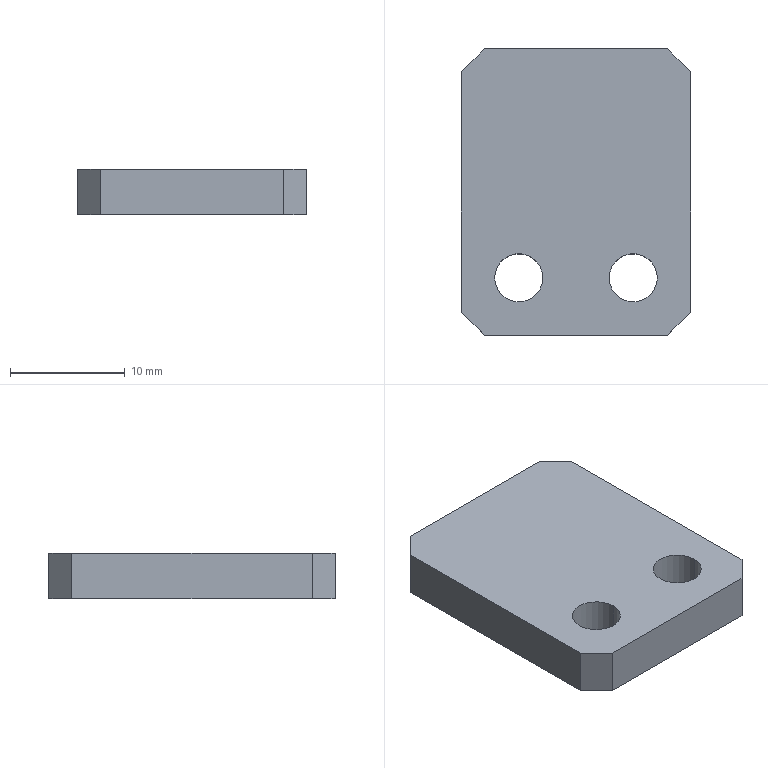Part | STEP file | PN_0085 Mount electronic clip slider stop plate | 1 solid | 14 faces | box 20 x 25 x 4 mm | volume 1857 mm3 | plane 10 | cylinder 4 | commonest cylinder face diameters 4.2 x4
STEP:
#1=CARTESIAN_POINT('',(0.,0.,0.));
#2=DIRECTION('',(0.,0.,1.));
#3=DIRECTION('',(1.,0.,0.));
#4=AXIS2_PLACEMENT_3D('',#1,#2,#3);
#5=CARTESIAN_POINT('',(-2.9,-7.5,0.));
#6=VERTEX_POINT('',#5);
#7=CARTESIAN_POINT('',(-2.9,-7.5,4.));
#8=VERTEX_POINT('',#7);
#9=CARTESIAN_POINT('',(-2.9,-7.5,4.));
#10=DIRECTION('',(0.,0.,1.));
#11=VECTOR('',#10,1.);
#12=LINE('',#9,#11);
#13=CARTESIAN_POINT('',(-5.,-7.5,4.));
#14=DIRECTION('',(0.,0.,1.));
#15=DIRECTION('',(1.,0.,0.));
#16=AXIS2_PLACEMENT_3D('',#13,#14,#15);
#17=CYLINDRICAL_SURFACE('',#16,2.1);
#18=CARTESIAN_POINT('',(6.283,0.));
#19=DIRECTION('',(0.,1.));
#20=VECTOR('',#19,1.);
#21=LINE('',#18,#20);
#22=(GEOMETRIC_REPRESENTATION_CONTEXT(2)PARAMETRIC_REPRESENTATION_CONTEXT()REPRESENTATION_CONTEXT('',''));
#23=DEFINITIONAL_REPRESENTATION('',(#21),#22);
#24=PCURVE('',#17,#23);
#25=CARTESIAN_POINT('',(-5.,-7.5,4.));
#26=DIRECTION('',(0.,0.,1.));
#27=DIRECTION('',(1.,0.,0.));
#28=AXIS2_PLACEMENT_3D('',#25,#26,#27);
#29=CYLINDRICAL_SURFACE('',#28,2.1);
#30=CARTESIAN_POINT('',(0.,0.));
#31=DIRECTION('',(0.,1.));
#32=VECTOR('',#31,1.);
#33=LINE('',#30,#32);
#34=(GEOMETRIC_REPRESENTATION_CONTEXT(2)PARAMETRIC_REPRESENTATION_CONTEXT()REPRESENTATION_CONTEXT('',''));
#35=DEFINITIONAL_REPRESENTATION('',(#33),#34);
#36=PCURVE('',#29,#35);
#37=SURFACE_CURVE('',#12,(#24,#36),.PCURVE_S1.);
#38=EDGE_CURVE('',#6,#8,#37,.T.);
#39=ORIENTED_EDGE('',*,*,#38,.T.);
#40=CARTESIAN_POINT('',(-7.1,-7.5,4.));
#41=VERTEX_POINT('',#40);
#42=CARTESIAN_POINT('',(-5.,-7.5,4.));
#43=DIRECTION('',(0.,0.,1.));
#44=DIRECTION('',(1.,0.,0.));
#45=AXIS2_PLACEMENT_3D('',#42,#43,#44);
#46=CIRCLE('',#45,2.1);
#47=CARTESIAN_POINT('',(0.,0.));
#48=DIRECTION('',(1.,0.));
#49=VECTOR('',#48,1.);
#50=LINE('',#47,#49);
#51=(GEOMETRIC_REPRESENTATION_CONTEXT(2)PARAMETRIC_REPRESENTATION_CONTEXT()REPRESENTATION_CONTEXT('',''));
#52=DEFINITIONAL_REPRESENTATION('',(#50),#51);
#53=PCURVE('',#17,#52);
#54=CARTESIAN_POINT('',(0.,0.,4.));
#55=DIRECTION('',(0.,0.,-1.));
#56=DIRECTION('',(-1.,0.,0.));
#57=AXIS2_PLACEMENT_3D('',#54,#55,#56);
#58=PLANE('',#57);
#59=CARTESIAN_POINT('',(2.9,-7.5));
#60=CARTESIAN_POINT('',(2.9,-3.863));
#61=CARTESIAN_POINT('',(6.05,-5.681));
#62=CARTESIAN_POINT('',(9.2,-7.5));
#63=CARTESIAN_POINT('',(6.05,-9.319));
#64=CARTESIAN_POINT('',(2.9,-11.137));
#65=CARTESIAN_POINT('',(2.9,-7.5));
#66=(BOUNDED_CURVE()B_SPLINE_CURVE(2,(#59,#60,#61,#62,#63,#64,#65),.UNSPECIFIED.,.T.,.F.)B_SPLINE_CURVE_WITH_KNOTS((1,2,2,2,2,1),(-2.094,0.,2.094,4.189,6.283,8.378),.UNSPECIFIED.)CURVE()GEOMETRIC_REPRESENTATION_ITEM()RATIONAL_B_SPLINE_CURVE((1.,0.5,1.,0.5,1.,0.5,1.))REPRESENTATION_ITEM(''));
#67=(GEOMETRIC_REPRESENTATION_CONTEXT(2)PARAMETRIC_REPRESENTATION_CONTEXT()REPRESENTATION_CONTEXT('',''));
#68=DEFINITIONAL_REPRESENTATION('',(#66),#67);
#69=PCURVE('',#58,#68);
#70=SURFACE_CURVE('',#46,(#53,#69),.PCURVE_S1.);
#71=EDGE_CURVE('',#41,#8,#70,.T.);
#72=ORIENTED_EDGE('',*,*,#71,.F.);
#73=CARTESIAN_POINT('',(-7.1,-7.5,0.));
#74=VERTEX_POINT('',#73);
#75=CARTESIAN_POINT('',(-7.1,-7.5,4.));
#76=DIRECTION('',(0.,0.,1.));
#77=VECTOR('',#76,1.);
#78=LINE('',#75,#77);
#79=CARTESIAN_POINT('',(3.142,0.));
#80=DIRECTION('',(0.,1.));
#81=VECTOR('',#80,1.);
#82=LINE('',#79,#81);
#83=(GEOMETRIC_REPRESENTATION_CONTEXT(2)PARAMETRIC_REPRESENTATION_CONTEXT()REPRESENTATION_CONTEXT('',''));
#84=DEFINITIONAL_REPRESENTATION('',(#82),#83);
#85=PCURVE('',#17,#84);
#86=CARTESIAN_POINT('',(3.142,0.));
#87=DIRECTION('',(0.,1.));
#88=VECTOR('',#87,1.);
#89=LINE('',#86,#88);
#90=(GEOMETRIC_REPRESENTATION_CONTEXT(2)PARAMETRIC_REPRESENTATION_CONTEXT()REPRESENTATION_CONTEXT('',''));
#91=DEFINITIONAL_REPRESENTATION('',(#89),#90);
#92=PCURVE('',#29,#91);
#93=SURFACE_CURVE('',#78,(#85,#92),.PCURVE_S1.);
#94=EDGE_CURVE('',#74,#41,#93,.T.);
#95=ORIENTED_EDGE('',*,*,#94,.F.);
#96=CARTESIAN_POINT('',(-5.,-7.5,0.));
#97=DIRECTION('',(0.,0.,-1.));
#98=DIRECTION('',(-1.,0.,0.));
#99=AXIS2_PLACEMENT_3D('',#96,#97,#98);
#100=CIRCLE('',#99,2.1);
#101=CARTESIAN_POINT('',(9.425,-4.));
#102=DIRECTION('',(-1.,0.));
#103=VECTOR('',#102,1.);
#104=LINE('',#101,#103);
#105=(GEOMETRIC_REPRESENTATION_CONTEXT(2)PARAMETRIC_REPRESENTATION_CONTEXT()REPRESENTATION_CONTEXT('',''));
#106=DEFINITIONAL_REPRESENTATION('',(#104),#105);
#107=PCURVE('',#17,#106);
#108=CARTESIAN_POINT('',(0.,0.,0.));
#109=DIRECTION('',(0.,0.,-1.));
#110=DIRECTION('',(-1.,0.,0.));
#111=AXIS2_PLACEMENT_3D('',#108,#109,#110);
#112=PLANE('',#111);
#113=CARTESIAN_POINT('',(5.,-7.5));
#114=DIRECTION('',(1.,0.));
#115=AXIS2_PLACEMENT_2D('',#113,#114);
#116=CIRCLE('',#115,2.1);
#117=(GEOMETRIC_REPRESENTATION_CONTEXT(2)PARAMETRIC_REPRESENTATION_CONTEXT()REPRESENTATION_CONTEXT('',''));
#118=DEFINITIONAL_REPRESENTATION('',(#116),#117);
#119=PCURVE('',#112,#118);
#120=SURFACE_CURVE('',#100,(#107,#119),.PCURVE_S1.);
#121=EDGE_CURVE('',#6,#74,#120,.T.);
#122=ORIENTED_EDGE('',*,*,#121,.F.);
#123=EDGE_LOOP('',(#39,#72,#95,#122));
#124=FACE_BOUND('',#123,.F.);
#125=ADVANCED_FACE('',(#124),#17,.F.);
#126=CARTESIAN_POINT('',(7.1,-7.5,0.));
#127=VERTEX_POINT('',#126);
#128=CARTESIAN_POINT('',(7.1,-7.5,4.));
#129=VERTEX_POINT('',#128);
#130=CARTESIAN_POINT('',(7.1,-7.5,4.));
#131=DIRECTION('',(0.,0.,1.));
#132=VECTOR('',#131,1.);
#133=LINE('',#130,#132);
#134=CARTESIAN_POINT('',(5.,-7.5,4.));
#135=DIRECTION('',(0.,0.,1.));
#136=DIRECTION('',(1.,0.,0.));
#137=AXIS2_PLACEMENT_3D('',#134,#135,#136);
#138=CYLINDRICAL_SURFACE('',#137,2.1);
#139=CARTESIAN_POINT('',(6.283,0.));
#140=DIRECTION('',(0.,1.));
#141=VECTOR('',#140,1.);
#142=LINE('',#139,#141);
#143=(GEOMETRIC_REPRESENTATION_CONTEXT(2)PARAMETRIC_REPRESENTATION_CONTEXT()REPRESENTATION_CONTEXT('',''));
#144=DEFINITIONAL_REPRESENTATION('',(#142),#143);
#145=PCURVE('',#138,#144);
#146=CARTESIAN_POINT('',(5.,-7.5,4.));
#147=DIRECTION('',(0.,0.,1.));
#148=DIRECTION('',(1.,0.,0.));
#149=AXIS2_PLACEMENT_3D('',#146,#147,#148);
#150=CYLINDRICAL_SURFACE('',#149,2.1);
#151=CARTESIAN_POINT('',(0.,0.));
#152=DIRECTION('',(0.,1.));
#153=VECTOR('',#152,1.);
#154=LINE('',#151,#153);
#155=(GEOMETRIC_REPRESENTATION_CONTEXT(2)PARAMETRIC_REPRESENTATION_CONTEXT()REPRESENTATION_CONTEXT('',''));
#156=DEFINITIONAL_REPRESENTATION('',(#154),#155);
#157=PCURVE('',#150,#156);
#158=SURFACE_CURVE('',#133,(#145,#157),.PCURVE_S1.);
#159=EDGE_CURVE('',#127,#129,#158,.T.);
#160=ORIENTED_EDGE('',*,*,#159,.T.);
#161=CARTESIAN_POINT('',(2.9,-7.5,4.));
#162=VERTEX_POINT('',#161);
#163=CARTESIAN_POINT('',(5.,-7.5,4.));
#164=DIRECTION('',(0.,0.,1.));
#165=DIRECTION('',(1.,0.,0.));
#166=AXIS2_PLACEMENT_3D('',#163,#164,#165);
#167=CIRCLE('',#166,2.1);
#168=CARTESIAN_POINT('',(0.,0.));
#169=DIRECTION('',(1.,0.));
#170=VECTOR('',#169,1.);
#171=LINE('',#168,#170);
#172=(GEOMETRIC_REPRESENTATION_CONTEXT(2)PARAMETRIC_REPRESENTATION_CONTEXT()REPRESENTATION_CONTEXT('',''));
#173=DEFINITIONAL_REPRESENTATION('',(#171),#172);
#174=PCURVE('',#138,#173);
#175=CARTESIAN_POINT('',(-7.1,-7.5));
#176=CARTESIAN_POINT('',(-7.1,-3.863));
#177=CARTESIAN_POINT('',(-3.95,-5.681));
#178=CARTESIAN_POINT('',(-0.8,-7.5));
#179=CARTESIAN_POINT('',(-3.95,-9.319));
#180=CARTESIAN_POINT('',(-7.1,-11.137));
#181=CARTESIAN_POINT('',(-7.1,-7.5));
#182=(BOUNDED_CURVE()B_SPLINE_CURVE(2,(#175,#176,#177,#178,#179,#180,#181),.UNSPECIFIED.,.T.,.F.)B_SPLINE_CURVE_WITH_KNOTS((1,2,2,2,2,1),(-2.094,0.,2.094,4.189,6.283,8.378),.UNSPECIFIED.)CURVE()GEOMETRIC_REPRESENTATION_ITEM()RATIONAL_B_SPLINE_CURVE((1.,0.5,1.,0.5,1.,0.5,1.))REPRESENTATION_ITEM(''));
#183=(GEOMETRIC_REPRESENTATION_CONTEXT(2)PARAMETRIC_REPRESENTATION_CONTEXT()REPRESENTATION_CONTEXT('',''));
#184=DEFINITIONAL_REPRESENTATION('',(#182),#183);
#185=PCURVE('',#58,#184);
#186=SURFACE_CURVE('',#167,(#174,#185),.PCURVE_S1.);
#187=EDGE_CURVE('',#162,#129,#186,.T.);
#188=ORIENTED_EDGE('',*,*,#187,.F.);
#189=CARTESIAN_POINT('',(2.9,-7.5,0.));
#190=VERTEX_POINT('',#189);
#191=CARTESIAN_POINT('',(2.9,-7.5,4.));
#192=DIRECTION('',(0.,0.,1.));
#193=VECTOR('',#192,1.);
#194=LINE('',#191,#193);
#195=CARTESIAN_POINT('',(3.142,0.));
#196=DIRECTION('',(0.,1.));
#197=VECTOR('',#196,1.);
#198=LINE('',#195,#197);
#199=(GEOMETRIC_REPRESENTATION_CONTEXT(2)PARAMETRIC_REPRESENTATION_CONTEXT()REPRESENTATION_CONTEXT('',''));
#200=DEFINITIONAL_REPRESENTATION('',(#198),#199);
#201=PCURVE('',#138,#200);
#202=CARTESIAN_POINT('',(3.142,0.));
#203=DIRECTION('',(0.,1.));
#204=VECTOR('',#203,1.);
#205=LINE('',#202,#204);
#206=(GEOMETRIC_REPRESENTATION_CONTEXT(2)PARAMETRIC_REPRESENTATION_CONTEXT()REPRESENTATION_CONTEXT('',''));
#207=DEFINITIONAL_REPRESENTATION('',(#205),#206);
#208=PCURVE('',#150,#207);
#209=SURFACE_CURVE('',#194,(#201,#208),.PCURVE_S1.);
#210=EDGE_CURVE('',#190,#162,#209,.T.);
#211=ORIENTED_EDGE('',*,*,#210,.F.);
#212=CARTESIAN_POINT('',(5.,-7.5,0.));
#213=DIRECTION('',(0.,0.,-1.));
#214=DIRECTION('',(-1.,0.,0.));
#215=AXIS2_PLACEMENT_3D('',#212,#213,#214);
#216=CIRCLE('',#215,2.1);
#217=CARTESIAN_POINT('',(9.425,-4.));
#218=DIRECTION('',(-1.,0.));
#219=VECTOR('',#218,1.);
#220=LINE('',#217,#219);
#221=(GEOMETRIC_REPRESENTATION_CONTEXT(2)PARAMETRIC_REPRESENTATION_CONTEXT()REPRESENTATION_CONTEXT('',''));
#222=DEFINITIONAL_REPRESENTATION('',(#220),#221);
#223=PCURVE('',#138,#222);
#224=CARTESIAN_POINT('',(-5.,-7.5));
#225=DIRECTION('',(1.,0.));
#226=AXIS2_PLACEMENT_2D('',#224,#225);
#227=CIRCLE('',#226,2.1);
#228=(GEOMETRIC_REPRESENTATION_CONTEXT(2)PARAMETRIC_REPRESENTATION_CONTEXT()REPRESENTATION_CONTEXT('',''));
#229=DEFINITIONAL_REPRESENTATION('',(#227),#228);
#230=PCURVE('',#112,#229);
#231=SURFACE_CURVE('',#216,(#223,#230),.PCURVE_S1.);
#232=EDGE_CURVE('',#127,#190,#231,.T.);
#233=ORIENTED_EDGE('',*,*,#232,.F.);
#234=EDGE_LOOP('',(#160,#188,#211,#233));
#235=FACE_BOUND('',#234,.F.);
#236=ADVANCED_FACE('',(#235),#138,.F.);
#237=CARTESIAN_POINT('',(10.,-10.5,4.));
#238=VERTEX_POINT('',#237);
#239=CARTESIAN_POINT('',(10.,10.5,4.));
#240=VERTEX_POINT('',#239);
#241=CARTESIAN_POINT('',(10.,-12.5,4.));
#242=DIRECTION('',(0.,1.,0.));
#243=VECTOR('',#242,1.);
#244=LINE('',#241,#243);
#245=CARTESIAN_POINT('',(10.,-12.5,4.));
#246=DIRECTION('',(-1.,0.,0.));
#247=DIRECTION('',(0.,0.,1.));
#248=AXIS2_PLACEMENT_3D('',#245,#246,#247);
#249=PLANE('',#248);
#250=CARTESIAN_POINT('',(0.,0.));
#251=DIRECTION('',(0.,1.));
#252=VECTOR('',#251,1.);
#253=LINE('',#250,#252);
#254=(GEOMETRIC_REPRESENTATION_CONTEXT(2)PARAMETRIC_REPRESENTATION_CONTEXT()REPRESENTATION_CONTEXT('',''));
#255=DEFINITIONAL_REPRESENTATION('',(#253),#254);
#256=PCURVE('',#249,#255);
#257=CARTESIAN_POINT('',(-10.,-12.5));
#258=DIRECTION('',(0.,1.));
#259=VECTOR('',#258,1.);
#260=LINE('',#257,#259);
#261=(GEOMETRIC_REPRESENTATION_CONTEXT(2)PARAMETRIC_REPRESENTATION_CONTEXT()REPRESENTATION_CONTEXT('',''));
#262=DEFINITIONAL_REPRESENTATION('',(#260),#261);
#263=PCURVE('',#58,#262);
#264=SURFACE_CURVE('',#244,(#256,#263),.PCURVE_S1.);
#265=EDGE_CURVE('',#238,#240,#264,.T.);
#266=ORIENTED_EDGE('',*,*,#265,.F.);
#267=CARTESIAN_POINT('',(10.,-10.5,0.));
#268=VERTEX_POINT('',#267);
#269=CARTESIAN_POINT('',(10.,-10.5,4.));
#270=DIRECTION('',(0.,0.,-1.));
#271=VECTOR('',#270,1.);
#272=LINE('',#269,#271);
#273=CARTESIAN_POINT('',(0.,2.));
#274=DIRECTION('',(-1.,0.));
#275=VECTOR('',#274,1.);
#276=LINE('',#273,#275);
#277=(GEOMETRIC_REPRESENTATION_CONTEXT(2)PARAMETRIC_REPRESENTATION_CONTEXT()REPRESENTATION_CONTEXT('',''));
#278=DEFINITIONAL_REPRESENTATION('',(#276),#277);
#279=PCURVE('',#249,#278);
#280=CARTESIAN_POINT('',(10.,-10.5,4.));
#281=DIRECTION('',(-0.7071,0.7071,0.));
#282=DIRECTION('',(0.,0.,-1.));
#283=AXIS2_PLACEMENT_3D('',#280,#281,#282);
#284=PLANE('',#283);
#285=CARTESIAN_POINT('',(0.,0.));
#286=DIRECTION('',(1.,0.));
#287=VECTOR('',#286,1.);
#288=LINE('',#285,#287);
#289=(GEOMETRIC_REPRESENTATION_CONTEXT(2)PARAMETRIC_REPRESENTATION_CONTEXT()REPRESENTATION_CONTEXT('',''));
#290=DEFINITIONAL_REPRESENTATION('',(#288),#289);
#291=PCURVE('',#284,#290);
#292=SURFACE_CURVE('',#272,(#279,#291),.PCURVE_S1.);
#293=EDGE_CURVE('',#238,#268,#292,.T.);
#294=ORIENTED_EDGE('',*,*,#293,.T.);
#295=CARTESIAN_POINT('',(10.,10.5,0.));
#296=VERTEX_POINT('',#295);
#297=CARTESIAN_POINT('',(10.,-12.5,0.));
#298=DIRECTION('',(0.,1.,0.));
#299=VECTOR('',#298,1.);
#300=LINE('',#297,#299);
#301=CARTESIAN_POINT('',(-4.,0.));
#302=DIRECTION('',(0.,1.));
#303=VECTOR('',#302,1.);
#304=LINE('',#301,#303);
#305=(GEOMETRIC_REPRESENTATION_CONTEXT(2)PARAMETRIC_REPRESENTATION_CONTEXT()REPRESENTATION_CONTEXT('',''));
#306=DEFINITIONAL_REPRESENTATION('',(#304),#305);
#307=PCURVE('',#249,#306);
#308=CARTESIAN_POINT('',(-10.,-12.5));
#309=DIRECTION('',(0.,1.));
#310=VECTOR('',#309,1.);
#311=LINE('',#308,#310);
#312=(GEOMETRIC_REPRESENTATION_CONTEXT(2)PARAMETRIC_REPRESENTATION_CONTEXT()REPRESENTATION_CONTEXT('',''));
#313=DEFINITIONAL_REPRESENTATION('',(#311),#312);
#314=PCURVE('',#112,#313);
#315=SURFACE_CURVE('',#300,(#307,#314),.PCURVE_S1.);
#316=EDGE_CURVE('',#268,#296,#315,.T.);
#317=ORIENTED_EDGE('',*,*,#316,.T.);
#318=CARTESIAN_POINT('',(10.,10.5,4.));
#319=DIRECTION('',(0.,0.,1.));
#320=VECTOR('',#319,1.);
#321=LINE('',#318,#320);
#322=CARTESIAN_POINT('',(0.,23.));
#323=DIRECTION('',(1.,0.));
#324=VECTOR('',#323,1.);
#325=LINE('',#322,#324);
#326=(GEOMETRIC_REPRESENTATION_CONTEXT(2)PARAMETRIC_REPRESENTATION_CONTEXT()REPRESENTATION_CONTEXT('',''));
#327=DEFINITIONAL_REPRESENTATION('',(#325),#326);
#328=PCURVE('',#249,#327);
#329=CARTESIAN_POINT('',(8.,12.5,4.));
#330=DIRECTION('',(-0.7071,-0.7071,0.));
#331=DIRECTION('',(0.,0.,-1.));
#332=AXIS2_PLACEMENT_3D('',#329,#330,#331);
#333=PLANE('',#332);
#334=CARTESIAN_POINT('',(0.,2.828));
#335=DIRECTION('',(-1.,0.));
#336=VECTOR('',#335,1.);
#337=LINE('',#334,#336);
#338=(GEOMETRIC_REPRESENTATION_CONTEXT(2)PARAMETRIC_REPRESENTATION_CONTEXT()REPRESENTATION_CONTEXT('',''));
#339=DEFINITIONAL_REPRESENTATION('',(#337),#338);
#340=PCURVE('',#333,#339);
#341=SURFACE_CURVE('',#321,(#328,#340),.PCURVE_S1.);
#342=EDGE_CURVE('',#296,#240,#341,.T.);
#343=ORIENTED_EDGE('',*,*,#342,.T.);
#344=EDGE_LOOP('',(#266,#294,#317,#343));
#345=FACE_BOUND('',#344,.T.);
#346=ADVANCED_FACE('',(#345),#249,.F.);
#347=CARTESIAN_POINT('',(8.,12.5,4.));
#348=VERTEX_POINT('',#347);
#349=CARTESIAN_POINT('',(-8.,12.5,4.));
#350=VERTEX_POINT('',#349);
#351=CARTESIAN_POINT('',(-10.,12.5,4.));
#352=DIRECTION('',(-1.,0.,0.));
#353=VECTOR('',#352,1.);
#354=LINE('',#351,#353);
#355=CARTESIAN_POINT('',(-10.,12.5,4.));
#356=DIRECTION('',(0.,-1.,0.));
#357=DIRECTION('',(0.,0.,-1.));
#358=AXIS2_PLACEMENT_3D('',#355,#356,#357);
#359=PLANE('',#358);
#360=CARTESIAN_POINT('',(0.,0.));
#361=DIRECTION('',(0.,-1.));
#362=VECTOR('',#361,1.);
#363=LINE('',#360,#362);
#364=(GEOMETRIC_REPRESENTATION_CONTEXT(2)PARAMETRIC_REPRESENTATION_CONTEXT()REPRESENTATION_CONTEXT('',''));
#365=DEFINITIONAL_REPRESENTATION('',(#363),#364);
#366=PCURVE('',#359,#365);
#367=CARTESIAN_POINT('',(10.,12.5));
#368=DIRECTION('',(1.,0.));
#369=VECTOR('',#368,1.);
#370=LINE('',#367,#369);
#371=(GEOMETRIC_REPRESENTATION_CONTEXT(2)PARAMETRIC_REPRESENTATION_CONTEXT()REPRESENTATION_CONTEXT('',''));
#372=DEFINITIONAL_REPRESENTATION('',(#370),#371);
#373=PCURVE('',#58,#372);
#374=SURFACE_CURVE('',#354,(#366,#373),.PCURVE_S1.);
#375=EDGE_CURVE('',#348,#350,#374,.T.);
#376=ORIENTED_EDGE('',*,*,#375,.F.);
#377=CARTESIAN_POINT('',(8.,12.5,0.));
#378=VERTEX_POINT('',#377);
#379=CARTESIAN_POINT('',(8.,12.5,4.));
#380=DIRECTION('',(0.,0.,-1.));
#381=VECTOR('',#380,1.);
#382=LINE('',#379,#381);
#383=CARTESIAN_POINT('',(0.,18.));
#384=DIRECTION('',(1.,0.));
#385=VECTOR('',#384,1.);
#386=LINE('',#383,#385);
#387=(GEOMETRIC_REPRESENTATION_CONTEXT(2)PARAMETRIC_REPRESENTATION_CONTEXT()REPRESENTATION_CONTEXT('',''));
#388=DEFINITIONAL_REPRESENTATION('',(#386),#387);
#389=PCURVE('',#359,#388);
#390=CARTESIAN_POINT('',(0.,0.));
#391=DIRECTION('',(1.,0.));
#392=VECTOR('',#391,1.);
#393=LINE('',#390,#392);
#394=(GEOMETRIC_REPRESENTATION_CONTEXT(2)PARAMETRIC_REPRESENTATION_CONTEXT()REPRESENTATION_CONTEXT('',''));
#395=DEFINITIONAL_REPRESENTATION('',(#393),#394);
#396=PCURVE('',#333,#395);
#397=SURFACE_CURVE('',#382,(#389,#396),.PCURVE_S1.);
#398=EDGE_CURVE('',#348,#378,#397,.T.);
#399=ORIENTED_EDGE('',*,*,#398,.T.);
#400=CARTESIAN_POINT('',(-8.,12.5,0.));
#401=VERTEX_POINT('',#400);
#402=CARTESIAN_POINT('',(-10.,12.5,0.));
#403=DIRECTION('',(-1.,0.,0.));
#404=VECTOR('',#403,1.);
#405=LINE('',#402,#404);
#406=CARTESIAN_POINT('',(4.,0.));
#407=DIRECTION('',(0.,-1.));
#408=VECTOR('',#407,1.);
#409=LINE('',#406,#408);
#410=(GEOMETRIC_REPRESENTATION_CONTEXT(2)PARAMETRIC_REPRESENTATION_CONTEXT()REPRESENTATION_CONTEXT('',''));
#411=DEFINITIONAL_REPRESENTATION('',(#409),#410);
#412=PCURVE('',#359,#411);
#413=CARTESIAN_POINT('',(10.,12.5));
#414=DIRECTION('',(1.,0.));
#415=VECTOR('',#414,1.);
#416=LINE('',#413,#415);
#417=(GEOMETRIC_REPRESENTATION_CONTEXT(2)PARAMETRIC_REPRESENTATION_CONTEXT()REPRESENTATION_CONTEXT('',''));
#418=DEFINITIONAL_REPRESENTATION('',(#416),#417);
#419=PCURVE('',#112,#418);
#420=SURFACE_CURVE('',#405,(#412,#419),.PCURVE_S1.);
#421=EDGE_CURVE('',#378,#401,#420,.T.);
#422=ORIENTED_EDGE('',*,*,#421,.T.);
#423=CARTESIAN_POINT('',(-8.,12.5,4.));
#424=DIRECTION('',(0.,0.,1.));
#425=VECTOR('',#424,1.);
#426=LINE('',#423,#425);
#427=CARTESIAN_POINT('',(0.,2.));
#428=DIRECTION('',(-1.,0.));
#429=VECTOR('',#428,1.);
#430=LINE('',#427,#429);
#431=(GEOMETRIC_REPRESENTATION_CONTEXT(2)PARAMETRIC_REPRESENTATION_CONTEXT()REPRESENTATION_CONTEXT('',''));
#432=DEFINITIONAL_REPRESENTATION('',(#430),#431);
#433=PCURVE('',#359,#432);
#434=CARTESIAN_POINT('',(-10.,10.5,4.));
#435=DIRECTION('',(0.7071,-0.7071,0.));
#436=DIRECTION('',(0.,0.,-1.));
#437=AXIS2_PLACEMENT_3D('',#434,#435,#436);
#438=PLANE('',#437);
#439=CARTESIAN_POINT('',(0.,2.828));
#440=DIRECTION('',(-1.,0.));
#441=VECTOR('',#440,1.);
#442=LINE('',#439,#441);
#443=(GEOMETRIC_REPRESENTATION_CONTEXT(2)PARAMETRIC_REPRESENTATION_CONTEXT()REPRESENTATION_CONTEXT('',''));
#444=DEFINITIONAL_REPRESENTATION('',(#442),#443);
#445=PCURVE('',#438,#444);
#446=SURFACE_CURVE('',#426,(#433,#445),.PCURVE_S1.);
#447=EDGE_CURVE('',#401,#350,#446,.T.);
#448=ORIENTED_EDGE('',*,*,#447,.T.);
#449=EDGE_LOOP('',(#376,#399,#422,#448));
#450=FACE_BOUND('',#449,.T.);
#451=ADVANCED_FACE('',(#450),#359,.F.);
#452=CARTESIAN_POINT('',(-10.,10.5,0.));
#453=VERTEX_POINT('',#452);
#454=CARTESIAN_POINT('',(-10.,-10.5,0.));
#455=VERTEX_POINT('',#454);
#456=CARTESIAN_POINT('',(-10.,-12.5,0.));
#457=DIRECTION('',(0.,-1.,0.));
#458=VECTOR('',#457,1.);
#459=LINE('',#456,#458);
#460=CARTESIAN_POINT('',(-10.,-12.5,4.));
#461=DIRECTION('',(1.,0.,0.));
#462=DIRECTION('',(0.,0.,-1.));
#463=AXIS2_PLACEMENT_3D('',#460,#461,#462);
#464=PLANE('',#463);
#465=CARTESIAN_POINT('',(4.,0.));
#466=DIRECTION('',(0.,-1.));
#467=VECTOR('',#466,1.);
#468=LINE('',#465,#467);
#469=(GEOMETRIC_REPRESENTATION_CONTEXT(2)PARAMETRIC_REPRESENTATION_CONTEXT()REPRESENTATION_CONTEXT('',''));
#470=DEFINITIONAL_REPRESENTATION('',(#468),#469);
#471=PCURVE('',#464,#470);
#472=CARTESIAN_POINT('',(10.,-12.5));
#473=DIRECTION('',(0.,-1.));
#474=VECTOR('',#473,1.);
#475=LINE('',#472,#474);
#476=(GEOMETRIC_REPRESENTATION_CONTEXT(2)PARAMETRIC_REPRESENTATION_CONTEXT()REPRESENTATION_CONTEXT('',''));
#477=DEFINITIONAL_REPRESENTATION('',(#475),#476);
#478=PCURVE('',#112,#477);
#479=SURFACE_CURVE('',#459,(#471,#478),.PCURVE_S1.);
#480=EDGE_CURVE('',#453,#455,#479,.T.);
#481=ORIENTED_EDGE('',*,*,#480,.T.);
#482=CARTESIAN_POINT('',(-10.,-10.5,4.));
#483=VERTEX_POINT('',#482);
#484=CARTESIAN_POINT('',(-10.,-10.5,4.));
#485=DIRECTION('',(0.,0.,1.));
#486=VECTOR('',#485,1.);
#487=LINE('',#484,#486);
#488=CARTESIAN_POINT('',(0.,2.));
#489=DIRECTION('',(-1.,0.));
#490=VECTOR('',#489,1.);
#491=LINE('',#488,#490);
#492=(GEOMETRIC_REPRESENTATION_CONTEXT(2)PARAMETRIC_REPRESENTATION_CONTEXT()REPRESENTATION_CONTEXT('',''));
#493=DEFINITIONAL_REPRESENTATION('',(#491),#492);
#494=PCURVE('',#464,#493);
#495=CARTESIAN_POINT('',(-8.,-12.5,4.));
#496=DIRECTION('',(0.7071,0.7071,0.));
#497=DIRECTION('',(0.,0.,-1.));
#498=AXIS2_PLACEMENT_3D('',#495,#496,#497);
#499=PLANE('',#498);
#500=CARTESIAN_POINT('',(0.,2.828));
#501=DIRECTION('',(-1.,0.));
#502=VECTOR('',#501,1.);
#503=LINE('',#500,#502);
#504=(GEOMETRIC_REPRESENTATION_CONTEXT(2)PARAMETRIC_REPRESENTATION_CONTEXT()REPRESENTATION_CONTEXT('',''));
#505=DEFINITIONAL_REPRESENTATION('',(#503),#504);
#506=PCURVE('',#499,#505);
#507=SURFACE_CURVE('',#487,(#494,#506),.PCURVE_S1.);
#508=EDGE_CURVE('',#455,#483,#507,.T.);
#509=ORIENTED_EDGE('',*,*,#508,.T.);
#510=CARTESIAN_POINT('',(-10.,10.5,4.));
#511=VERTEX_POINT('',#510);
#512=CARTESIAN_POINT('',(-10.,-12.5,4.));
#513=DIRECTION('',(0.,-1.,0.));
#514=VECTOR('',#513,1.);
#515=LINE('',#512,#514);
#516=CARTESIAN_POINT('',(0.,0.));
#517=DIRECTION('',(0.,-1.));
#518=VECTOR('',#517,1.);
#519=LINE('',#516,#518);
#520=(GEOMETRIC_REPRESENTATION_CONTEXT(2)PARAMETRIC_REPRESENTATION_CONTEXT()REPRESENTATION_CONTEXT('',''));
#521=DEFINITIONAL_REPRESENTATION('',(#519),#520);
#522=PCURVE('',#464,#521);
#523=CARTESIAN_POINT('',(10.,-12.5));
#524=DIRECTION('',(0.,-1.));
#525=VECTOR('',#524,1.);
#526=LINE('',#523,#525);
#527=(GEOMETRIC_REPRESENTATION_CONTEXT(2)PARAMETRIC_REPRESENTATION_CONTEXT()REPRESENTATION_CONTEXT('',''));
#528=DEFINITIONAL_REPRESENTATION('',(#526),#527);
#529=PCURVE('',#58,#528);
#530=SURFACE_CURVE('',#515,(#522,#529),.PCURVE_S1.);
#531=EDGE_CURVE('',#511,#483,#530,.T.);
#532=ORIENTED_EDGE('',*,*,#531,.F.);
#533=CARTESIAN_POINT('',(-10.,10.5,4.));
#534=DIRECTION('',(0.,0.,-1.));
#535=VECTOR('',#534,1.);
#536=LINE('',#533,#535);
#537=CARTESIAN_POINT('',(0.,23.));
#538=DIRECTION('',(1.,0.));
#539=VECTOR('',#538,1.);
#540=LINE('',#537,#539);
#541=(GEOMETRIC_REPRESENTATION_CONTEXT(2)PARAMETRIC_REPRESENTATION_CONTEXT()REPRESENTATION_CONTEXT('',''));
#542=DEFINITIONAL_REPRESENTATION('',(#540),#541);
#543=PCURVE('',#464,#542);
#544=CARTESIAN_POINT('',(0.,0.));
#545=DIRECTION('',(1.,0.));
#546=VECTOR('',#545,1.);
#547=LINE('',#544,#546);
#548=(GEOMETRIC_REPRESENTATION_CONTEXT(2)PARAMETRIC_REPRESENTATION_CONTEXT()REPRESENTATION_CONTEXT('',''));
#549=DEFINITIONAL_REPRESENTATION('',(#547),#548);
#550=PCURVE('',#438,#549);
#551=SURFACE_CURVE('',#536,(#543,#550),.PCURVE_S1.);
#552=EDGE_CURVE('',#511,#453,#551,.T.);
#553=ORIENTED_EDGE('',*,*,#552,.T.);
#554=EDGE_LOOP('',(#481,#509,#532,#553));
#555=FACE_BOUND('',#554,.T.);
#556=ADVANCED_FACE('',(#555),#464,.F.);
#557=CARTESIAN_POINT('',(-8.,-12.5,0.));
#558=VERTEX_POINT('',#557);
#559=CARTESIAN_POINT('',(8.,-12.5,0.));
#560=VERTEX_POINT('',#559);
#561=CARTESIAN_POINT('',(-10.,-12.5,0.));
#562=DIRECTION('',(1.,0.,0.));
#563=VECTOR('',#562,1.);
#564=LINE('',#561,#563);
#565=CARTESIAN_POINT('',(-10.,-12.5,4.));
#566=DIRECTION('',(0.,1.,0.));
#567=DIRECTION('',(0.,0.,1.));
#568=AXIS2_PLACEMENT_3D('',#565,#566,#567);
#569=PLANE('',#568);
#570=CARTESIAN_POINT('',(-4.,0.));
#571=DIRECTION('',(0.,1.));
#572=VECTOR('',#571,1.);
#573=LINE('',#570,#572);
#574=(GEOMETRIC_REPRESENTATION_CONTEXT(2)PARAMETRIC_REPRESENTATION_CONTEXT()REPRESENTATION_CONTEXT('',''));
#575=DEFINITIONAL_REPRESENTATION('',(#573),#574);
#576=PCURVE('',#569,#575);
#577=CARTESIAN_POINT('',(10.,-12.5));
#578=DIRECTION('',(-1.,0.));
#579=VECTOR('',#578,1.);
#580=LINE('',#577,#579);
#581=(GEOMETRIC_REPRESENTATION_CONTEXT(2)PARAMETRIC_REPRESENTATION_CONTEXT()REPRESENTATION_CONTEXT('',''));
#582=DEFINITIONAL_REPRESENTATION('',(#580),#581);
#583=PCURVE('',#112,#582);
#584=SURFACE_CURVE('',#564,(#576,#583),.PCURVE_S1.);
#585=EDGE_CURVE('',#558,#560,#584,.T.);
#586=ORIENTED_EDGE('',*,*,#585,.T.);
#587=CARTESIAN_POINT('',(8.,-12.5,4.));
#588=VERTEX_POINT('',#587);
#589=CARTESIAN_POINT('',(8.,-12.5,4.));
#590=DIRECTION('',(0.,0.,1.));
#591=VECTOR('',#590,1.);
#592=LINE('',#589,#591);
#593=CARTESIAN_POINT('',(0.,18.));
#594=DIRECTION('',(1.,0.));
#595=VECTOR('',#594,1.);
#596=LINE('',#593,#595);
#597=(GEOMETRIC_REPRESENTATION_CONTEXT(2)PARAMETRIC_REPRESENTATION_CONTEXT()REPRESENTATION_CONTEXT('',''));
#598=DEFINITIONAL_REPRESENTATION('',(#596),#597);
#599=PCURVE('',#569,#598);
#600=CARTESIAN_POINT('',(0.,2.828));
#601=DIRECTION('',(-1.,0.));
#602=VECTOR('',#601,1.);
#603=LINE('',#600,#602);
#604=(GEOMETRIC_REPRESENTATION_CONTEXT(2)PARAMETRIC_REPRESENTATION_CONTEXT()REPRESENTATION_CONTEXT('',''));
#605=DEFINITIONAL_REPRESENTATION('',(#603),#604);
#606=PCURVE('',#284,#605);
#607=SURFACE_CURVE('',#592,(#599,#606),.PCURVE_S1.);
#608=EDGE_CURVE('',#560,#588,#607,.T.);
#609=ORIENTED_EDGE('',*,*,#608,.T.);
#610=CARTESIAN_POINT('',(-8.,-12.5,4.));
#611=VERTEX_POINT('',#610);
#612=CARTESIAN_POINT('',(-10.,-12.5,4.));
#613=DIRECTION('',(1.,0.,0.));
#614=VECTOR('',#613,1.);
#615=LINE('',#612,#614);
#616=CARTESIAN_POINT('',(0.,0.));
#617=DIRECTION('',(0.,1.));
#618=VECTOR('',#617,1.);
#619=LINE('',#616,#618);
#620=(GEOMETRIC_REPRESENTATION_CONTEXT(2)PARAMETRIC_REPRESENTATION_CONTEXT()REPRESENTATION_CONTEXT('',''));
#621=DEFINITIONAL_REPRESENTATION('',(#619),#620);
#622=PCURVE('',#569,#621);
#623=CARTESIAN_POINT('',(10.,-12.5));
#624=DIRECTION('',(-1.,0.));
#625=VECTOR('',#624,1.);
#626=LINE('',#623,#625);
#627=(GEOMETRIC_REPRESENTATION_CONTEXT(2)PARAMETRIC_REPRESENTATION_CONTEXT()REPRESENTATION_CONTEXT('',''));
#628=DEFINITIONAL_REPRESENTATION('',(#626),#627);
#629=PCURVE('',#58,#628);
#630=SURFACE_CURVE('',#615,(#622,#629),.PCURVE_S1.);
#631=EDGE_CURVE('',#611,#588,#630,.T.);
#632=ORIENTED_EDGE('',*,*,#631,.F.);
#633=CARTESIAN_POINT('',(-8.,-12.5,4.));
#634=DIRECTION('',(0.,0.,-1.));
#635=VECTOR('',#634,1.);
#636=LINE('',#633,#635);
#637=CARTESIAN_POINT('',(0.,2.));
#638=DIRECTION('',(-1.,0.));
#639=VECTOR('',#638,1.);
#640=LINE('',#637,#639);
#641=(GEOMETRIC_REPRESENTATION_CONTEXT(2)PARAMETRIC_REPRESENTATION_CONTEXT()REPRESENTATION_CONTEXT('',''));
#642=DEFINITIONAL_REPRESENTATION('',(#640),#641);
#643=PCURVE('',#569,#642);
#644=CARTESIAN_POINT('',(0.,0.));
#645=DIRECTION('',(1.,0.));
#646=VECTOR('',#645,1.);
#647=LINE('',#644,#646);
#648=(GEOMETRIC_REPRESENTATION_CONTEXT(2)PARAMETRIC_REPRESENTATION_CONTEXT()REPRESENTATION_CONTEXT('',''));
#649=DEFINITIONAL_REPRESENTATION('',(#647),#648);
#650=PCURVE('',#499,#649);
#651=SURFACE_CURVE('',#636,(#643,#650),.PCURVE_S1.);
#652=EDGE_CURVE('',#611,#558,#651,.T.);
#653=ORIENTED_EDGE('',*,*,#652,.T.);
#654=EDGE_LOOP('',(#586,#609,#632,#653));
#655=FACE_BOUND('',#654,.T.);
#656=ADVANCED_FACE('',(#655),#569,.F.);
#657=CARTESIAN_POINT('',(-5.,-7.5,4.));
#658=DIRECTION('',(0.,0.,1.));
#659=DIRECTION('',(1.,0.,0.));
#660=AXIS2_PLACEMENT_3D('',#657,#658,#659);
#661=CIRCLE('',#660,2.1);
#662=CARTESIAN_POINT('',(2.9,-7.5));
#663=CARTESIAN_POINT('',(2.9,-3.863));
#664=CARTESIAN_POINT('',(6.05,-5.681));
#665=CARTESIAN_POINT('',(9.2,-7.5));
#666=CARTESIAN_POINT('',(6.05,-9.319));
#667=CARTESIAN_POINT('',(2.9,-11.137));
#668=CARTESIAN_POINT('',(2.9,-7.5));
#669=(BOUNDED_CURVE()B_SPLINE_CURVE(2,(#662,#663,#664,#665,#666,#667,#668),.UNSPECIFIED.,.T.,.F.)B_SPLINE_CURVE_WITH_KNOTS((1,2,2,2,2,1),(-2.094,0.,2.094,4.189,6.283,8.378),.UNSPECIFIED.)CURVE()GEOMETRIC_REPRESENTATION_ITEM()RATIONAL_B_SPLINE_CURVE((1.,0.5,1.,0.5,1.,0.5,1.))REPRESENTATION_ITEM(''));
#670=(GEOMETRIC_REPRESENTATION_CONTEXT(2)PARAMETRIC_REPRESENTATION_CONTEXT()REPRESENTATION_CONTEXT('',''));
#671=DEFINITIONAL_REPRESENTATION('',(#669),#670);
#672=PCURVE('',#58,#671);
#673=CARTESIAN_POINT('',(0.,0.));
#674=DIRECTION('',(1.,0.));
#675=VECTOR('',#674,1.);
#676=LINE('',#673,#675);
#677=(GEOMETRIC_REPRESENTATION_CONTEXT(2)PARAMETRIC_REPRESENTATION_CONTEXT()REPRESENTATION_CONTEXT('',''));
#678=DEFINITIONAL_REPRESENTATION('',(#676),#677);
#679=PCURVE('',#29,#678);
#680=SURFACE_CURVE('',#661,(#672,#679),.PCURVE_S1.);
#681=EDGE_CURVE('',#8,#41,#680,.T.);
#682=ORIENTED_EDGE('',*,*,#681,.F.);
#683=ORIENTED_EDGE('',*,*,#71,.F.);
#684=EDGE_LOOP('',(#682,#683));
#685=FACE_BOUND('',#684,.T.);
#686=CARTESIAN_POINT('',(5.,-7.5,4.));
#687=DIRECTION('',(0.,0.,1.));
#688=DIRECTION('',(1.,0.,0.));
#689=AXIS2_PLACEMENT_3D('',#686,#687,#688);
#690=CIRCLE('',#689,2.1);
#691=CARTESIAN_POINT('',(-7.1,-7.5));
#692=CARTESIAN_POINT('',(-7.1,-3.863));
#693=CARTESIAN_POINT('',(-3.95,-5.681));
#694=CARTESIAN_POINT('',(-0.8,-7.5));
#695=CARTESIAN_POINT('',(-3.95,-9.319));
#696=CARTESIAN_POINT('',(-7.1,-11.137));
#697=CARTESIAN_POINT('',(-7.1,-7.5));
#698=(BOUNDED_CURVE()B_SPLINE_CURVE(2,(#691,#692,#693,#694,#695,#696,#697),.UNSPECIFIED.,.T.,.F.)B_SPLINE_CURVE_WITH_KNOTS((1,2,2,2,2,1),(-2.094,0.,2.094,4.189,6.283,8.378),.UNSPECIFIED.)CURVE()GEOMETRIC_REPRESENTATION_ITEM()RATIONAL_B_SPLINE_CURVE((1.,0.5,1.,0.5,1.,0.5,1.))REPRESENTATION_ITEM(''));
#699=(GEOMETRIC_REPRESENTATION_CONTEXT(2)PARAMETRIC_REPRESENTATION_CONTEXT()REPRESENTATION_CONTEXT('',''));
#700=DEFINITIONAL_REPRESENTATION('',(#698),#699);
#701=PCURVE('',#58,#700);
#702=CARTESIAN_POINT('',(0.,0.));
#703=DIRECTION('',(1.,0.));
#704=VECTOR('',#703,1.);
#705=LINE('',#702,#704);
#706=(GEOMETRIC_REPRESENTATION_CONTEXT(2)PARAMETRIC_REPRESENTATION_CONTEXT()REPRESENTATION_CONTEXT('',''));
#707=DEFINITIONAL_REPRESENTATION('',(#705),#706);
#708=PCURVE('',#150,#707);
#709=SURFACE_CURVE('',#690,(#701,#708),.PCURVE_S1.);
#710=EDGE_CURVE('',#129,#162,#709,.T.);
#711=ORIENTED_EDGE('',*,*,#710,.F.);
#712=ORIENTED_EDGE('',*,*,#187,.F.);
#713=EDGE_LOOP('',(#711,#712));
#714=FACE_BOUND('',#713,.T.);
#715=ORIENTED_EDGE('',*,*,#631,.T.);
#716=CARTESIAN_POINT('',(10.,-10.5,4.));
#717=DIRECTION('',(0.7071,0.7071,0.));
#718=VECTOR('',#717,1.);
#719=LINE('',#716,#718);
#720=CARTESIAN_POINT('',(-10.,-10.5));
#721=DIRECTION('',(-0.7071,0.7071));
#722=VECTOR('',#721,1.);
#723=LINE('',#720,#722);
#724=(GEOMETRIC_REPRESENTATION_CONTEXT(2)PARAMETRIC_REPRESENTATION_CONTEXT()REPRESENTATION_CONTEXT('',''));
#725=DEFINITIONAL_REPRESENTATION('',(#723),#724);
#726=PCURVE('',#58,#725);
#727=CARTESIAN_POINT('',(0.,0.));
#728=DIRECTION('',(0.,-1.));
#729=VECTOR('',#728,1.);
#730=LINE('',#727,#729);
#731=(GEOMETRIC_REPRESENTATION_CONTEXT(2)PARAMETRIC_REPRESENTATION_CONTEXT()REPRESENTATION_CONTEXT('',''));
#732=DEFINITIONAL_REPRESENTATION('',(#730),#731);
#733=PCURVE('',#284,#732);
#734=SURFACE_CURVE('',#719,(#726,#733),.PCURVE_S1.);
#735=EDGE_CURVE('',#588,#238,#734,.T.);
#736=ORIENTED_EDGE('',*,*,#735,.T.);
#737=ORIENTED_EDGE('',*,*,#265,.T.);
#738=CARTESIAN_POINT('',(8.,12.5,4.));
#739=DIRECTION('',(-0.7071,0.7071,0.));
#740=VECTOR('',#739,1.);
#741=LINE('',#738,#740);
#742=CARTESIAN_POINT('',(-8.,12.5));
#743=DIRECTION('',(0.7071,0.7071));
#744=VECTOR('',#743,1.);
#745=LINE('',#742,#744);
#746=(GEOMETRIC_REPRESENTATION_CONTEXT(2)PARAMETRIC_REPRESENTATION_CONTEXT()REPRESENTATION_CONTEXT('',''));
#747=DEFINITIONAL_REPRESENTATION('',(#745),#746);
#748=PCURVE('',#58,#747);
#749=CARTESIAN_POINT('',(0.,0.));
#750=DIRECTION('',(0.,-1.));
#751=VECTOR('',#750,1.);
#752=LINE('',#749,#751);
#753=(GEOMETRIC_REPRESENTATION_CONTEXT(2)PARAMETRIC_REPRESENTATION_CONTEXT()REPRESENTATION_CONTEXT('',''));
#754=DEFINITIONAL_REPRESENTATION('',(#752),#753);
#755=PCURVE('',#333,#754);
#756=SURFACE_CURVE('',#741,(#748,#755),.PCURVE_S1.);
#757=EDGE_CURVE('',#240,#348,#756,.T.);
#758=ORIENTED_EDGE('',*,*,#757,.T.);
#759=ORIENTED_EDGE('',*,*,#375,.T.);
#760=CARTESIAN_POINT('',(-10.,10.5,4.));
#761=DIRECTION('',(-0.7071,-0.7071,0.));
#762=VECTOR('',#761,1.);
#763=LINE('',#760,#762);
#764=CARTESIAN_POINT('',(10.,10.5));
#765=DIRECTION('',(0.7071,-0.7071));
#766=VECTOR('',#765,1.);
#767=LINE('',#764,#766);
#768=(GEOMETRIC_REPRESENTATION_CONTEXT(2)PARAMETRIC_REPRESENTATION_CONTEXT()REPRESENTATION_CONTEXT('',''));
#769=DEFINITIONAL_REPRESENTATION('',(#767),#768);
#770=PCURVE('',#58,#769);
#771=CARTESIAN_POINT('',(0.,0.));
#772=DIRECTION('',(0.,-1.));
#773=VECTOR('',#772,1.);
#774=LINE('',#771,#773);
#775=(GEOMETRIC_REPRESENTATION_CONTEXT(2)PARAMETRIC_REPRESENTATION_CONTEXT()REPRESENTATION_CONTEXT('',''));
#776=DEFINITIONAL_REPRESENTATION('',(#774),#775);
#777=PCURVE('',#438,#776);
#778=SURFACE_CURVE('',#763,(#770,#777),.PCURVE_S1.);
#779=EDGE_CURVE('',#350,#511,#778,.T.);
#780=ORIENTED_EDGE('',*,*,#779,.T.);
#781=ORIENTED_EDGE('',*,*,#531,.T.);
#782=CARTESIAN_POINT('',(-8.,-12.5,4.));
#783=DIRECTION('',(0.7071,-0.7071,0.));
#784=VECTOR('',#783,1.);
#785=LINE('',#782,#784);
#786=CARTESIAN_POINT('',(8.,-12.5));
#787=DIRECTION('',(-0.7071,-0.7071));
#788=VECTOR('',#787,1.);
#789=LINE('',#786,#788);
#790=(GEOMETRIC_REPRESENTATION_CONTEXT(2)PARAMETRIC_REPRESENTATION_CONTEXT()REPRESENTATION_CONTEXT('',''));
#791=DEFINITIONAL_REPRESENTATION('',(#789),#790);
#792=PCURVE('',#58,#791);
#793=CARTESIAN_POINT('',(0.,0.));
#794=DIRECTION('',(0.,-1.));
#795=VECTOR('',#794,1.);
#796=LINE('',#793,#795);
#797=(GEOMETRIC_REPRESENTATION_CONTEXT(2)PARAMETRIC_REPRESENTATION_CONTEXT()REPRESENTATION_CONTEXT('',''));
#798=DEFINITIONAL_REPRESENTATION('',(#796),#797);
#799=PCURVE('',#499,#798);
#800=SURFACE_CURVE('',#785,(#792,#799),.PCURVE_S1.);
#801=EDGE_CURVE('',#483,#611,#800,.T.);
#802=ORIENTED_EDGE('',*,*,#801,.T.);
#803=EDGE_LOOP('',(#715,#736,#737,#758,#759,#780,#781,#802));
#804=FACE_BOUND('',#803,.T.);
#805=ADVANCED_FACE('',(#685,#714,#804),#58,.F.);
#806=ORIENTED_EDGE('',*,*,#121,.F.);
#807=CARTESIAN_POINT('',(-5.,-7.5,0.));
#808=DIRECTION('',(0.,0.,-1.));
#809=DIRECTION('',(-1.,0.,0.));
#810=AXIS2_PLACEMENT_3D('',#807,#808,#809);
#811=CIRCLE('',#810,2.1);
#812=CARTESIAN_POINT('',(5.,-7.5));
#813=DIRECTION('',(1.,0.));
#814=AXIS2_PLACEMENT_2D('',#812,#813);
#815=CIRCLE('',#814,2.1);
#816=(GEOMETRIC_REPRESENTATION_CONTEXT(2)PARAMETRIC_REPRESENTATION_CONTEXT()REPRESENTATION_CONTEXT('',''));
#817=DEFINITIONAL_REPRESENTATION('',(#815),#816);
#818=PCURVE('',#112,#817);
#819=CARTESIAN_POINT('',(3.142,-4.));
#820=DIRECTION('',(-1.,0.));
#821=VECTOR('',#820,1.);
#822=LINE('',#819,#821);
#823=(GEOMETRIC_REPRESENTATION_CONTEXT(2)PARAMETRIC_REPRESENTATION_CONTEXT()REPRESENTATION_CONTEXT('',''));
#824=DEFINITIONAL_REPRESENTATION('',(#822),#823);
#825=PCURVE('',#29,#824);
#826=SURFACE_CURVE('',#811,(#818,#825),.PCURVE_S1.);
#827=EDGE_CURVE('',#74,#6,#826,.T.);
#828=ORIENTED_EDGE('',*,*,#827,.F.);
#829=EDGE_LOOP('',(#806,#828));
#830=FACE_BOUND('',#829,.T.);
#831=ORIENTED_EDGE('',*,*,#232,.F.);
#832=CARTESIAN_POINT('',(5.,-7.5,0.));
#833=DIRECTION('',(0.,0.,-1.));
#834=DIRECTION('',(-1.,0.,0.));
#835=AXIS2_PLACEMENT_3D('',#832,#833,#834);
#836=CIRCLE('',#835,2.1);
#837=CARTESIAN_POINT('',(-5.,-7.5));
#838=DIRECTION('',(1.,0.));
#839=AXIS2_PLACEMENT_2D('',#837,#838);
#840=CIRCLE('',#839,2.1);
#841=(GEOMETRIC_REPRESENTATION_CONTEXT(2)PARAMETRIC_REPRESENTATION_CONTEXT()REPRESENTATION_CONTEXT('',''));
#842=DEFINITIONAL_REPRESENTATION('',(#840),#841);
#843=PCURVE('',#112,#842);
#844=CARTESIAN_POINT('',(3.142,-4.));
#845=DIRECTION('',(-1.,0.));
#846=VECTOR('',#845,1.);
#847=LINE('',#844,#846);
#848=(GEOMETRIC_REPRESENTATION_CONTEXT(2)PARAMETRIC_REPRESENTATION_CONTEXT()REPRESENTATION_CONTEXT('',''));
#849=DEFINITIONAL_REPRESENTATION('',(#847),#848);
#850=PCURVE('',#150,#849);
#851=SURFACE_CURVE('',#836,(#843,#850),.PCURVE_S1.);
#852=EDGE_CURVE('',#190,#127,#851,.T.);
#853=ORIENTED_EDGE('',*,*,#852,.F.);
#854=EDGE_LOOP('',(#831,#853));
#855=FACE_BOUND('',#854,.T.);
#856=ORIENTED_EDGE('',*,*,#316,.F.);
#857=CARTESIAN_POINT('',(10.25,-10.25,0.));
#858=DIRECTION('',(-0.7071,-0.7071,0.));
#859=VECTOR('',#858,1.);
#860=LINE('',#857,#859);
#861=CARTESIAN_POINT('',(-10.25,-10.25));
#862=DIRECTION('',(0.7071,-0.7071));
#863=VECTOR('',#862,1.);
#864=LINE('',#861,#863);
#865=(GEOMETRIC_REPRESENTATION_CONTEXT(2)PARAMETRIC_REPRESENTATION_CONTEXT()REPRESENTATION_CONTEXT('',''));
#866=DEFINITIONAL_REPRESENTATION('',(#864),#865);
#867=PCURVE('',#112,#866);
#868=CARTESIAN_POINT('',(4.,-0.3536));
#869=DIRECTION('',(0.,1.));
#870=VECTOR('',#869,1.);
#871=LINE('',#868,#870);
#872=(GEOMETRIC_REPRESENTATION_CONTEXT(2)PARAMETRIC_REPRESENTATION_CONTEXT()REPRESENTATION_CONTEXT('',''));
#873=DEFINITIONAL_REPRESENTATION('',(#871),#872);
#874=PCURVE('',#284,#873);
#875=SURFACE_CURVE('',#860,(#867,#874),.PCURVE_S1.);
#876=EDGE_CURVE('',#268,#560,#875,.T.);
#877=ORIENTED_EDGE('',*,*,#876,.T.);
#878=ORIENTED_EDGE('',*,*,#585,.F.);
#879=CARTESIAN_POINT('',(-10.25,-10.25,0.));
#880=DIRECTION('',(-0.7071,0.7071,0.));
#881=VECTOR('',#880,1.);
#882=LINE('',#879,#881);
#883=CARTESIAN_POINT('',(10.25,-10.25));
#884=DIRECTION('',(0.7071,0.7071));
#885=VECTOR('',#884,1.);
#886=LINE('',#883,#885);
#887=(GEOMETRIC_REPRESENTATION_CONTEXT(2)PARAMETRIC_REPRESENTATION_CONTEXT()REPRESENTATION_CONTEXT('',''));
#888=DEFINITIONAL_REPRESENTATION('',(#886),#887);
#889=PCURVE('',#112,#888);
#890=CARTESIAN_POINT('',(4.,3.182));
#891=DIRECTION('',(0.,1.));
#892=VECTOR('',#891,1.);
#893=LINE('',#890,#892);
#894=(GEOMETRIC_REPRESENTATION_CONTEXT(2)PARAMETRIC_REPRESENTATION_CONTEXT()REPRESENTATION_CONTEXT('',''));
#895=DEFINITIONAL_REPRESENTATION('',(#893),#894);
#896=PCURVE('',#499,#895);
#897=SURFACE_CURVE('',#882,(#889,#896),.PCURVE_S1.);
#898=EDGE_CURVE('',#558,#455,#897,.T.);
#899=ORIENTED_EDGE('',*,*,#898,.T.);
#900=ORIENTED_EDGE('',*,*,#480,.F.);
#901=CARTESIAN_POINT('',(-10.25,10.25,0.));
#902=DIRECTION('',(0.7071,0.7071,0.));
#903=VECTOR('',#902,1.);
#904=LINE('',#901,#903);
#905=CARTESIAN_POINT('',(10.25,10.25));
#906=DIRECTION('',(-0.7071,0.7071));
#907=VECTOR('',#906,1.);
#908=LINE('',#905,#907);
#909=(GEOMETRIC_REPRESENTATION_CONTEXT(2)PARAMETRIC_REPRESENTATION_CONTEXT()REPRESENTATION_CONTEXT('',''));
#910=DEFINITIONAL_REPRESENTATION('',(#908),#909);
#911=PCURVE('',#112,#910);
#912=CARTESIAN_POINT('',(4.,-0.3536));
#913=DIRECTION('',(0.,1.));
#914=VECTOR('',#913,1.);
#915=LINE('',#912,#914);
#916=(GEOMETRIC_REPRESENTATION_CONTEXT(2)PARAMETRIC_REPRESENTATION_CONTEXT()REPRESENTATION_CONTEXT('',''));
#917=DEFINITIONAL_REPRESENTATION('',(#915),#916);
#918=PCURVE('',#438,#917);
#919=SURFACE_CURVE('',#904,(#911,#918),.PCURVE_S1.);
#920=EDGE_CURVE('',#453,#401,#919,.T.);
#921=ORIENTED_EDGE('',*,*,#920,.T.);
#922=ORIENTED_EDGE('',*,*,#421,.F.);
#923=CARTESIAN_POINT('',(10.25,10.25,0.));
#924=DIRECTION('',(0.7071,-0.7071,0.));
#925=VECTOR('',#924,1.);
#926=LINE('',#923,#925);
#927=CARTESIAN_POINT('',(-10.25,10.25));
#928=DIRECTION('',(-0.7071,-0.7071));
#929=VECTOR('',#928,1.);
#930=LINE('',#927,#929);
#931=(GEOMETRIC_REPRESENTATION_CONTEXT(2)PARAMETRIC_REPRESENTATION_CONTEXT()REPRESENTATION_CONTEXT('',''));
#932=DEFINITIONAL_REPRESENTATION('',(#930),#931);
#933=PCURVE('',#112,#932);
#934=CARTESIAN_POINT('',(4.,3.182));
#935=DIRECTION('',(0.,1.));
#936=VECTOR('',#935,1.);
#937=LINE('',#934,#936);
#938=(GEOMETRIC_REPRESENTATION_CONTEXT(2)PARAMETRIC_REPRESENTATION_CONTEXT()REPRESENTATION_CONTEXT('',''));
#939=DEFINITIONAL_REPRESENTATION('',(#937),#938);
#940=PCURVE('',#333,#939);
#941=SURFACE_CURVE('',#926,(#933,#940),.PCURVE_S1.);
#942=EDGE_CURVE('',#378,#296,#941,.T.);
#943=ORIENTED_EDGE('',*,*,#942,.T.);
#944=EDGE_LOOP('',(#856,#877,#878,#899,#900,#921,#922,#943));
#945=FACE_BOUND('',#944,.T.);
#946=ADVANCED_FACE('',(#830,#855,#945),#112,.T.);
#947=ORIENTED_EDGE('',*,*,#710,.F.);
#948=ORIENTED_EDGE('',*,*,#159,.F.);
#949=ORIENTED_EDGE('',*,*,#852,.F.);
#950=ORIENTED_EDGE('',*,*,#210,.T.);
#951=EDGE_LOOP('',(#947,#948,#949,#950));
#952=FACE_BOUND('',#951,.F.);
#953=ADVANCED_FACE('',(#952),#150,.F.);
#954=ORIENTED_EDGE('',*,*,#681,.F.);
#955=ORIENTED_EDGE('',*,*,#38,.F.);
#956=ORIENTED_EDGE('',*,*,#827,.F.);
#957=ORIENTED_EDGE('',*,*,#94,.T.);
#958=EDGE_LOOP('',(#954,#955,#956,#957));
#959=FACE_BOUND('',#958,.F.);
#960=ADVANCED_FACE('',(#959),#29,.F.);
#961=ORIENTED_EDGE('',*,*,#735,.F.);
#962=ORIENTED_EDGE('',*,*,#608,.F.);
#963=ORIENTED_EDGE('',*,*,#876,.F.);
#964=ORIENTED_EDGE('',*,*,#293,.F.);
#965=EDGE_LOOP('',(#961,#962,#963,#964));
#966=FACE_BOUND('',#965,.T.);
#967=ADVANCED_FACE('',(#966),#284,.F.);
#968=ORIENTED_EDGE('',*,*,#801,.F.);
#969=ORIENTED_EDGE('',*,*,#508,.F.);
#970=ORIENTED_EDGE('',*,*,#898,.F.);
#971=ORIENTED_EDGE('',*,*,#652,.F.);
#972=EDGE_LOOP('',(#968,#969,#970,#971));
#973=FACE_BOUND('',#972,.T.);
#974=ADVANCED_FACE('',(#973),#499,.F.);
#975=ORIENTED_EDGE('',*,*,#757,.F.);
#976=ORIENTED_EDGE('',*,*,#342,.F.);
#977=ORIENTED_EDGE('',*,*,#942,.F.);
#978=ORIENTED_EDGE('',*,*,#398,.F.);
#979=EDGE_LOOP('',(#975,#976,#977,#978));
#980=FACE_BOUND('',#979,.T.);
#981=ADVANCED_FACE('',(#980),#333,.F.);
#982=ORIENTED_EDGE('',*,*,#779,.F.);
#983=ORIENTED_EDGE('',*,*,#447,.F.);
#984=ORIENTED_EDGE('',*,*,#920,.F.);
#985=ORIENTED_EDGE('',*,*,#552,.F.);
#986=EDGE_LOOP('',(#982,#983,#984,#985));
#987=FACE_BOUND('',#986,.T.);
#988=ADVANCED_FACE('',(#987),#438,.F.);
#989=CLOSED_SHELL('',(#125,#236,#346,#451,#556,#656,#805,#946,#953,#960,#967,#974,#981,#988));
#990=MANIFOLD_SOLID_BREP('',#989);
#991=(LENGTH_UNIT()NAMED_UNIT(*)SI_UNIT(.MILLI.,.METRE.));
#992=UNCERTAINTY_MEASURE_WITH_UNIT(LENGTH_MEASURE(0.0000001),#991,'','');
#993=(NAMED_UNIT(*)PLANE_ANGLE_UNIT()SI_UNIT($,.RADIAN.));
#994=(NAMED_UNIT(*)SI_UNIT($,.STERADIAN.)SOLID_ANGLE_UNIT());
#995=(GEOMETRIC_REPRESENTATION_CONTEXT(3)GLOBAL_UNCERTAINTY_ASSIGNED_CONTEXT((#992))GLOBAL_UNIT_ASSIGNED_CONTEXT((#991,#993,#994))REPRESENTATION_CONTEXT('',''));
#996=ADVANCED_BREP_SHAPE_REPRESENTATION('',(#4,#990),#995);